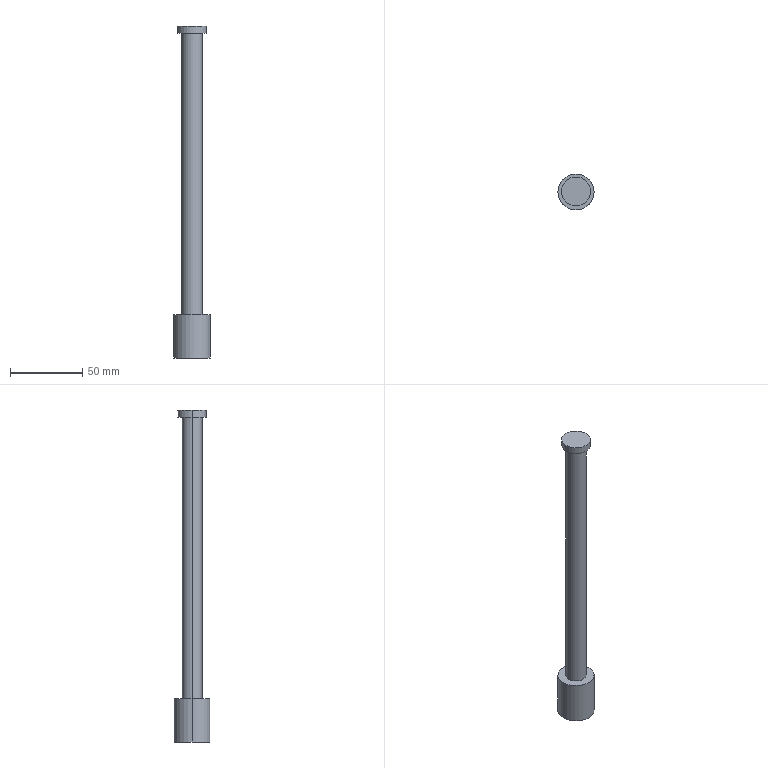Part | SolidWorks | 1 solid | 13 faces | box 25 x 25 x 230 mm | volume 40077 mm3 | cylinder 8 | plane 5 | commonest cylinder face diameters 14 x2 19 x2 20 x2 25 x2
STEP:
#1=CARTESIAN_POINT('',(9.5,0.,-105.5));
#2=VERTEX_POINT('',#1);
#3=CARTESIAN_POINT('',(-9.5,0.,-105.5));
#4=VERTEX_POINT('',#3);
#5=CARTESIAN_POINT('',(0.,0.,-105.5));
#6=DIRECTION('',(0.,0.,-1.));
#7=DIRECTION('',(-1.,0.,0.));
#8=AXIS2_PLACEMENT_3D('',#5,#6,#7);
#9=CIRCLE('',#8,9.5);
#10=EDGE_CURVE('',#2,#4,#9,.T.);
#11=ORIENTED_EDGE('',*,*,#10,.F.);
#12=CARTESIAN_POINT('',(9.5,0.,-127.5));
#13=VERTEX_POINT('',#12);
#14=CARTESIAN_POINT('',(9.5,0.,-105.5));
#15=DIRECTION('',(0.,0.,-1.));
#16=VECTOR('',#15,1000.);
#17=LINE('',#14,#16);
#18=EDGE_CURVE('',#2,#13,#17,.T.);
#19=ORIENTED_EDGE('',*,*,#18,.T.);
#20=CARTESIAN_POINT('',(-9.5,0.,-127.5));
#21=VERTEX_POINT('',#20);
#22=CARTESIAN_POINT('',(0.,0.,-127.5));
#23=DIRECTION('',(0.,0.,-1.));
#24=DIRECTION('',(-1.,0.,0.));
#25=AXIS2_PLACEMENT_3D('',#22,#23,#24);
#26=CIRCLE('',#25,9.5);
#27=EDGE_CURVE('',#13,#21,#26,.T.);
#28=ORIENTED_EDGE('',*,*,#27,.T.);
#29=CARTESIAN_POINT('',(-9.5,0.,-105.5));
#30=DIRECTION('',(0.,0.,-1.));
#31=VECTOR('',#30,1000.);
#32=LINE('',#29,#31);
#33=EDGE_CURVE('',#4,#21,#32,.T.);
#34=ORIENTED_EDGE('',*,*,#33,.F.);
#35=EDGE_LOOP('',(#11,#19,#28,#34));
#36=FACE_OUTER_BOUND('',#35,.T.);
#37=CARTESIAN_POINT('',(0.,0.,-105.5));
#38=DIRECTION('',(0.,0.,-1.));
#39=DIRECTION('',(-1.,0.,0.));
#40=AXIS2_PLACEMENT_3D('',#37,#38,#39);
#41=CYLINDRICAL_SURFACE('',#40,9.5);
#42=ADVANCED_FACE('',(#36),#41,.F.);
#43=CARTESIAN_POINT('',(-12.5,0.,-127.5));
#44=VERTEX_POINT('',#43);
#45=CARTESIAN_POINT('',(12.5,0.,-127.5));
#46=VERTEX_POINT('',#45);
#47=CARTESIAN_POINT('',(0.,0.,-127.5));
#48=DIRECTION('',(0.,0.,-1.));
#49=DIRECTION('',(-1.,0.,0.));
#50=AXIS2_PLACEMENT_3D('',#47,#48,#49);
#51=CIRCLE('',#50,12.5);
#52=EDGE_CURVE('',#44,#46,#51,.T.);
#53=ORIENTED_EDGE('',*,*,#52,.F.);
#54=CARTESIAN_POINT('',(-12.5,0.,-97.5));
#55=VERTEX_POINT('',#54);
#56=CARTESIAN_POINT('',(-12.5,0.,-127.5));
#57=DIRECTION('',(0.,0.,1.));
#58=VECTOR('',#57,1000.);
#59=LINE('',#56,#58);
#60=EDGE_CURVE('',#44,#55,#59,.T.);
#61=ORIENTED_EDGE('',*,*,#60,.T.);
#62=CARTESIAN_POINT('',(12.5,0.,-97.5));
#63=VERTEX_POINT('',#62);
#64=CARTESIAN_POINT('',(0.,0.,-97.5));
#65=DIRECTION('',(0.,0.,-1.));
#66=DIRECTION('',(-1.,0.,0.));
#67=AXIS2_PLACEMENT_3D('',#64,#65,#66);
#68=CIRCLE('',#67,12.5);
#69=EDGE_CURVE('',#55,#63,#68,.T.);
#70=ORIENTED_EDGE('',*,*,#69,.T.);
#71=CARTESIAN_POINT('',(12.5,0.,-127.5));
#72=DIRECTION('',(0.,0.,1.));
#73=VECTOR('',#72,1000.);
#74=LINE('',#71,#73);
#75=EDGE_CURVE('',#46,#63,#74,.T.);
#76=ORIENTED_EDGE('',*,*,#75,.F.);
#77=EDGE_LOOP('',(#53,#61,#70,#76));
#78=FACE_OUTER_BOUND('',#77,.T.);
#79=CARTESIAN_POINT('',(0.,0.,-127.5));
#80=DIRECTION('',(0.,0.,1.));
#81=DIRECTION('',(1.,0.,0.));
#82=AXIS2_PLACEMENT_3D('',#79,#80,#81);
#83=CYLINDRICAL_SURFACE('',#82,12.5);
#84=ADVANCED_FACE('',(#78),#83,.T.);
#85=CARTESIAN_POINT('',(10.,0.,102.5));
#86=VERTEX_POINT('',#85);
#87=CARTESIAN_POINT('',(-10.,0.,102.5));
#88=VERTEX_POINT('',#87);
#89=CARTESIAN_POINT('',(0.,0.,102.5));
#90=DIRECTION('',(0.,0.,1.));
#91=DIRECTION('',(1.,0.,0.));
#92=AXIS2_PLACEMENT_3D('',#89,#90,#91);
#93=CIRCLE('',#92,10.);
#94=EDGE_CURVE('',#86,#88,#93,.T.);
#95=ORIENTED_EDGE('',*,*,#94,.F.);
#96=CARTESIAN_POINT('',(10.,0.,97.5));
#97=VERTEX_POINT('',#96);
#98=CARTESIAN_POINT('',(10.,0.,102.5));
#99=DIRECTION('',(0.,0.,-1.));
#100=VECTOR('',#99,1000.);
#101=LINE('',#98,#100);
#102=EDGE_CURVE('',#86,#97,#101,.T.);
#103=ORIENTED_EDGE('',*,*,#102,.T.);
#104=CARTESIAN_POINT('',(-10.,0.,97.5));
#105=VERTEX_POINT('',#104);
#106=CARTESIAN_POINT('',(0.,0.,97.5));
#107=DIRECTION('',(0.,0.,1.));
#108=DIRECTION('',(1.,0.,0.));
#109=AXIS2_PLACEMENT_3D('',#106,#107,#108);
#110=CIRCLE('',#109,10.);
#111=EDGE_CURVE('',#97,#105,#110,.T.);
#112=ORIENTED_EDGE('',*,*,#111,.T.);
#113=CARTESIAN_POINT('',(-10.,0.,102.5));
#114=DIRECTION('',(0.,0.,-1.));
#115=VECTOR('',#114,1000.);
#116=LINE('',#113,#115);
#117=EDGE_CURVE('',#88,#105,#116,.T.);
#118=ORIENTED_EDGE('',*,*,#117,.F.);
#119=EDGE_LOOP('',(#95,#103,#112,#118));
#120=FACE_OUTER_BOUND('',#119,.T.);
#121=CARTESIAN_POINT('',(0.,0.,102.5));
#122=DIRECTION('',(0.,0.,-1.));
#123=DIRECTION('',(-1.,0.,0.));
#124=AXIS2_PLACEMENT_3D('',#121,#122,#123);
#125=CYLINDRICAL_SURFACE('',#124,10.);
#126=ADVANCED_FACE('',(#120),#125,.T.);
#127=CARTESIAN_POINT('',(7.,0.,97.5));
#128=VERTEX_POINT('',#127);
#129=CARTESIAN_POINT('',(-7.,0.,97.5));
#130=VERTEX_POINT('',#129);
#131=CARTESIAN_POINT('',(0.,0.,97.5));
#132=DIRECTION('',(0.,0.,1.));
#133=DIRECTION('',(1.,0.,0.));
#134=AXIS2_PLACEMENT_3D('',#131,#132,#133);
#135=CIRCLE('',#134,7.);
#136=EDGE_CURVE('',#128,#130,#135,.T.);
#137=ORIENTED_EDGE('',*,*,#136,.F.);
#138=CARTESIAN_POINT('',(7.,0.,-97.5));
#139=VERTEX_POINT('',#138);
#140=CARTESIAN_POINT('',(7.,0.,97.5));
#141=DIRECTION('',(0.,0.,-1.));
#142=VECTOR('',#141,1000.);
#143=LINE('',#140,#142);
#144=EDGE_CURVE('',#128,#139,#143,.T.);
#145=ORIENTED_EDGE('',*,*,#144,.T.);
#146=CARTESIAN_POINT('',(-7.,0.,-97.5));
#147=VERTEX_POINT('',#146);
#148=CARTESIAN_POINT('',(0.,0.,-97.5));
#149=DIRECTION('',(0.,0.,1.));
#150=DIRECTION('',(1.,0.,0.));
#151=AXIS2_PLACEMENT_3D('',#148,#149,#150);
#152=CIRCLE('',#151,7.);
#153=EDGE_CURVE('',#139,#147,#152,.T.);
#154=ORIENTED_EDGE('',*,*,#153,.T.);
#155=CARTESIAN_POINT('',(-7.,0.,97.5));
#156=DIRECTION('',(0.,0.,-1.));
#157=VECTOR('',#156,1000.);
#158=LINE('',#155,#157);
#159=EDGE_CURVE('',#130,#147,#158,.T.);
#160=ORIENTED_EDGE('',*,*,#159,.F.);
#161=EDGE_LOOP('',(#137,#145,#154,#160));
#162=FACE_OUTER_BOUND('',#161,.T.);
#163=CARTESIAN_POINT('',(0.,0.,97.5));
#164=DIRECTION('',(0.,0.,-1.));
#165=DIRECTION('',(-1.,0.,0.));
#166=AXIS2_PLACEMENT_3D('',#163,#164,#165);
#167=CYLINDRICAL_SURFACE('',#166,7.);
#168=ADVANCED_FACE('',(#162),#167,.T.);
#169=ORIENTED_EDGE('',*,*,#144,.F.);
#170=CARTESIAN_POINT('',(0.,0.,97.5));
#171=DIRECTION('',(0.,0.,1.));
#172=DIRECTION('',(1.,0.,0.));
#173=AXIS2_PLACEMENT_3D('',#170,#171,#172);
#174=CIRCLE('',#173,7.);
#175=EDGE_CURVE('',#130,#128,#174,.T.);
#176=ORIENTED_EDGE('',*,*,#175,.F.);
#177=ORIENTED_EDGE('',*,*,#159,.T.);
#178=CARTESIAN_POINT('',(0.,0.,-97.5));
#179=DIRECTION('',(0.,0.,1.));
#180=DIRECTION('',(1.,0.,0.));
#181=AXIS2_PLACEMENT_3D('',#178,#179,#180);
#182=CIRCLE('',#181,7.);
#183=EDGE_CURVE('',#147,#139,#182,.T.);
#184=ORIENTED_EDGE('',*,*,#183,.T.);
#185=EDGE_LOOP('',(#169,#176,#177,#184));
#186=FACE_OUTER_BOUND('',#185,.T.);
#187=CARTESIAN_POINT('',(0.,0.,97.5));
#188=DIRECTION('',(0.,0.,-1.));
#189=DIRECTION('',(-1.,0.,0.));
#190=AXIS2_PLACEMENT_3D('',#187,#188,#189);
#191=CYLINDRICAL_SURFACE('',#190,7.);
#192=ADVANCED_FACE('',(#186),#191,.T.);
#193=ORIENTED_EDGE('',*,*,#102,.F.);
#194=CARTESIAN_POINT('',(0.,0.,102.5));
#195=DIRECTION('',(0.,0.,1.));
#196=DIRECTION('',(1.,0.,0.));
#197=AXIS2_PLACEMENT_3D('',#194,#195,#196);
#198=CIRCLE('',#197,10.);
#199=EDGE_CURVE('',#88,#86,#198,.T.);
#200=ORIENTED_EDGE('',*,*,#199,.F.);
#201=ORIENTED_EDGE('',*,*,#117,.T.);
#202=CARTESIAN_POINT('',(0.,0.,97.5));
#203=DIRECTION('',(0.,0.,1.));
#204=DIRECTION('',(1.,0.,0.));
#205=AXIS2_PLACEMENT_3D('',#202,#203,#204);
#206=CIRCLE('',#205,10.);
#207=EDGE_CURVE('',#105,#97,#206,.T.);
#208=ORIENTED_EDGE('',*,*,#207,.T.);
#209=EDGE_LOOP('',(#193,#200,#201,#208));
#210=FACE_OUTER_BOUND('',#209,.T.);
#211=CARTESIAN_POINT('',(0.,0.,102.5));
#212=DIRECTION('',(0.,0.,-1.));
#213=DIRECTION('',(-1.,0.,0.));
#214=AXIS2_PLACEMENT_3D('',#211,#212,#213);
#215=CYLINDRICAL_SURFACE('',#214,10.);
#216=ADVANCED_FACE('',(#210),#215,.T.);
#217=ORIENTED_EDGE('',*,*,#199,.T.);
#218=ORIENTED_EDGE('',*,*,#94,.T.);
#219=EDGE_LOOP('',(#217,#218));
#220=FACE_OUTER_BOUND('',#219,.T.);
#221=CARTESIAN_POINT('',(0.,0.,102.5));
#222=DIRECTION('',(0.,0.,1.));
#223=DIRECTION('',(1.,0.,0.));
#224=AXIS2_PLACEMENT_3D('',#221,#222,#223);
#225=PLANE('',#224);
#226=ADVANCED_FACE('',(#220),#225,.T.);
#227=ORIENTED_EDGE('',*,*,#175,.T.);
#228=ORIENTED_EDGE('',*,*,#136,.T.);
#229=EDGE_LOOP('',(#227,#228));
#230=FACE_BOUND('',#229,.T.);
#231=ORIENTED_EDGE('',*,*,#207,.F.);
#232=ORIENTED_EDGE('',*,*,#111,.F.);
#233=EDGE_LOOP('',(#231,#232));
#234=FACE_OUTER_BOUND('',#233,.T.);
#235=CARTESIAN_POINT('',(0.,0.,97.5));
#236=DIRECTION('',(0.,0.,1.));
#237=DIRECTION('',(1.,0.,0.));
#238=AXIS2_PLACEMENT_3D('',#235,#236,#237);
#239=PLANE('',#238);
#240=ADVANCED_FACE('',(#230,#234),#239,.F.);
#241=ORIENTED_EDGE('',*,*,#60,.F.);
#242=CARTESIAN_POINT('',(0.,0.,-127.5));
#243=DIRECTION('',(0.,0.,-1.));
#244=DIRECTION('',(-1.,0.,0.));
#245=AXIS2_PLACEMENT_3D('',#242,#243,#244);
#246=CIRCLE('',#245,12.5);
#247=EDGE_CURVE('',#46,#44,#246,.T.);
#248=ORIENTED_EDGE('',*,*,#247,.F.);
#249=ORIENTED_EDGE('',*,*,#75,.T.);
#250=CARTESIAN_POINT('',(0.,0.,-97.5));
#251=DIRECTION('',(0.,0.,-1.));
#252=DIRECTION('',(-1.,0.,0.));
#253=AXIS2_PLACEMENT_3D('',#250,#251,#252);
#254=CIRCLE('',#253,12.5);
#255=EDGE_CURVE('',#63,#55,#254,.T.);
#256=ORIENTED_EDGE('',*,*,#255,.T.);
#257=EDGE_LOOP('',(#241,#248,#249,#256));
#258=FACE_OUTER_BOUND('',#257,.T.);
#259=CARTESIAN_POINT('',(0.,0.,-127.5));
#260=DIRECTION('',(0.,0.,1.));
#261=DIRECTION('',(1.,0.,0.));
#262=AXIS2_PLACEMENT_3D('',#259,#260,#261);
#263=CYLINDRICAL_SURFACE('',#262,12.5);
#264=ADVANCED_FACE('',(#258),#263,.T.);
#265=CARTESIAN_POINT('',(0.,0.,-127.5));
#266=DIRECTION('',(0.,0.,-1.));
#267=DIRECTION('',(-1.,0.,0.));
#268=AXIS2_PLACEMENT_3D('',#265,#266,#267);
#269=CIRCLE('',#268,9.5);
#270=EDGE_CURVE('',#21,#13,#269,.T.);
#271=ORIENTED_EDGE('',*,*,#270,.F.);
#272=ORIENTED_EDGE('',*,*,#27,.F.);
#273=EDGE_LOOP('',(#271,#272));
#274=FACE_BOUND('',#273,.T.);
#275=ORIENTED_EDGE('',*,*,#247,.T.);
#276=ORIENTED_EDGE('',*,*,#52,.T.);
#277=EDGE_LOOP('',(#275,#276));
#278=FACE_OUTER_BOUND('',#277,.T.);
#279=CARTESIAN_POINT('',(0.,0.,-127.5));
#280=DIRECTION('',(0.,0.,-1.));
#281=DIRECTION('',(-1.,0.,0.));
#282=AXIS2_PLACEMENT_3D('',#279,#280,#281);
#283=PLANE('',#282);
#284=ADVANCED_FACE('',(#274,#278),#283,.T.);
#285=ORIENTED_EDGE('',*,*,#183,.F.);
#286=ORIENTED_EDGE('',*,*,#153,.F.);
#287=EDGE_LOOP('',(#285,#286));
#288=FACE_BOUND('',#287,.T.);
#289=ORIENTED_EDGE('',*,*,#255,.F.);
#290=ORIENTED_EDGE('',*,*,#69,.F.);
#291=EDGE_LOOP('',(#289,#290));
#292=FACE_OUTER_BOUND('',#291,.T.);
#293=CARTESIAN_POINT('',(0.,0.,-97.5));
#294=DIRECTION('',(0.,0.,-1.));
#295=DIRECTION('',(-1.,0.,0.));
#296=AXIS2_PLACEMENT_3D('',#293,#294,#295);
#297=PLANE('',#296);
#298=ADVANCED_FACE('',(#288,#292),#297,.F.);
#299=ORIENTED_EDGE('',*,*,#18,.F.);
#300=CARTESIAN_POINT('',(0.,0.,-105.5));
#301=DIRECTION('',(0.,0.,-1.));
#302=DIRECTION('',(-1.,0.,0.));
#303=AXIS2_PLACEMENT_3D('',#300,#301,#302);
#304=CIRCLE('',#303,9.5);
#305=EDGE_CURVE('',#4,#2,#304,.T.);
#306=ORIENTED_EDGE('',*,*,#305,.F.);
#307=ORIENTED_EDGE('',*,*,#33,.T.);
#308=ORIENTED_EDGE('',*,*,#270,.T.);
#309=EDGE_LOOP('',(#299,#306,#307,#308));
#310=FACE_OUTER_BOUND('',#309,.T.);
#311=CARTESIAN_POINT('',(0.,0.,-105.5));
#312=DIRECTION('',(0.,0.,-1.));
#313=DIRECTION('',(-1.,0.,0.));
#314=AXIS2_PLACEMENT_3D('',#311,#312,#313);
#315=CYLINDRICAL_SURFACE('',#314,9.5);
#316=ADVANCED_FACE('',(#310),#315,.F.);
#317=ORIENTED_EDGE('',*,*,#305,.T.);
#318=ORIENTED_EDGE('',*,*,#10,.T.);
#319=EDGE_LOOP('',(#317,#318));
#320=FACE_OUTER_BOUND('',#319,.T.);
#321=CARTESIAN_POINT('',(0.,0.,-105.5));
#322=DIRECTION('',(0.,0.,-1.));
#323=DIRECTION('',(-1.,0.,0.));
#324=AXIS2_PLACEMENT_3D('',#321,#322,#323);
#325=PLANE('',#324);
#326=ADVANCED_FACE('',(#320),#325,.T.);
#327=CLOSED_SHELL('',(#42,#84,#126,#168,#192,#216,#226,#240,#264,#284,#298,#316,#326));
#328=MANIFOLD_SOLID_BREP('',#327);
#329=CARTESIAN_POINT('',(0.,0.,0.));
#330=DIRECTION('',(0.,0.,1.));
#331=DIRECTION('',(1.,0.,0.));
#332=AXIS2_PLACEMENT_3D('',#329,#330,#331);
#333=(LENGTH_UNIT()NAMED_UNIT(*)SI_UNIT(.MILLI.,.METRE.));
#334=UNCERTAINTY_MEASURE_WITH_UNIT(LENGTH_MEASURE(0.00001),#333,'','');
#335=(NAMED_UNIT(*)PLANE_ANGLE_UNIT()SI_UNIT($,.RADIAN.));
#336=(NAMED_UNIT(*)SI_UNIT($,.STERADIAN.)SOLID_ANGLE_UNIT());
#337=(GEOMETRIC_REPRESENTATION_CONTEXT(3)GLOBAL_UNCERTAINTY_ASSIGNED_CONTEXT((#334))GLOBAL_UNIT_ASSIGNED_CONTEXT((#333,#335,#336))REPRESENTATION_CONTEXT('',''));
#338=ADVANCED_BREP_SHAPE_REPRESENTATION('',(#328,#332),#337);